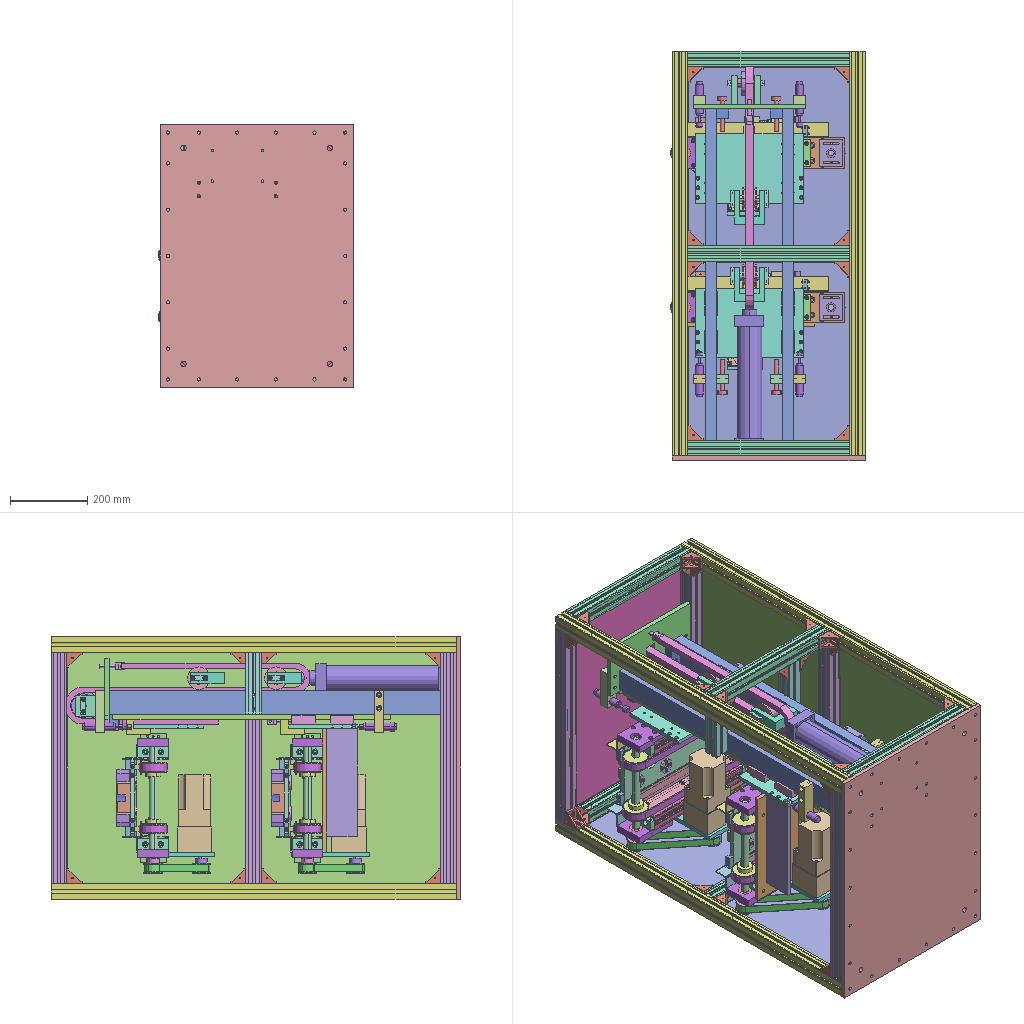Assembly | STEP file | 73 different items | 248 placed | box 503 x 1062 x 680 mm
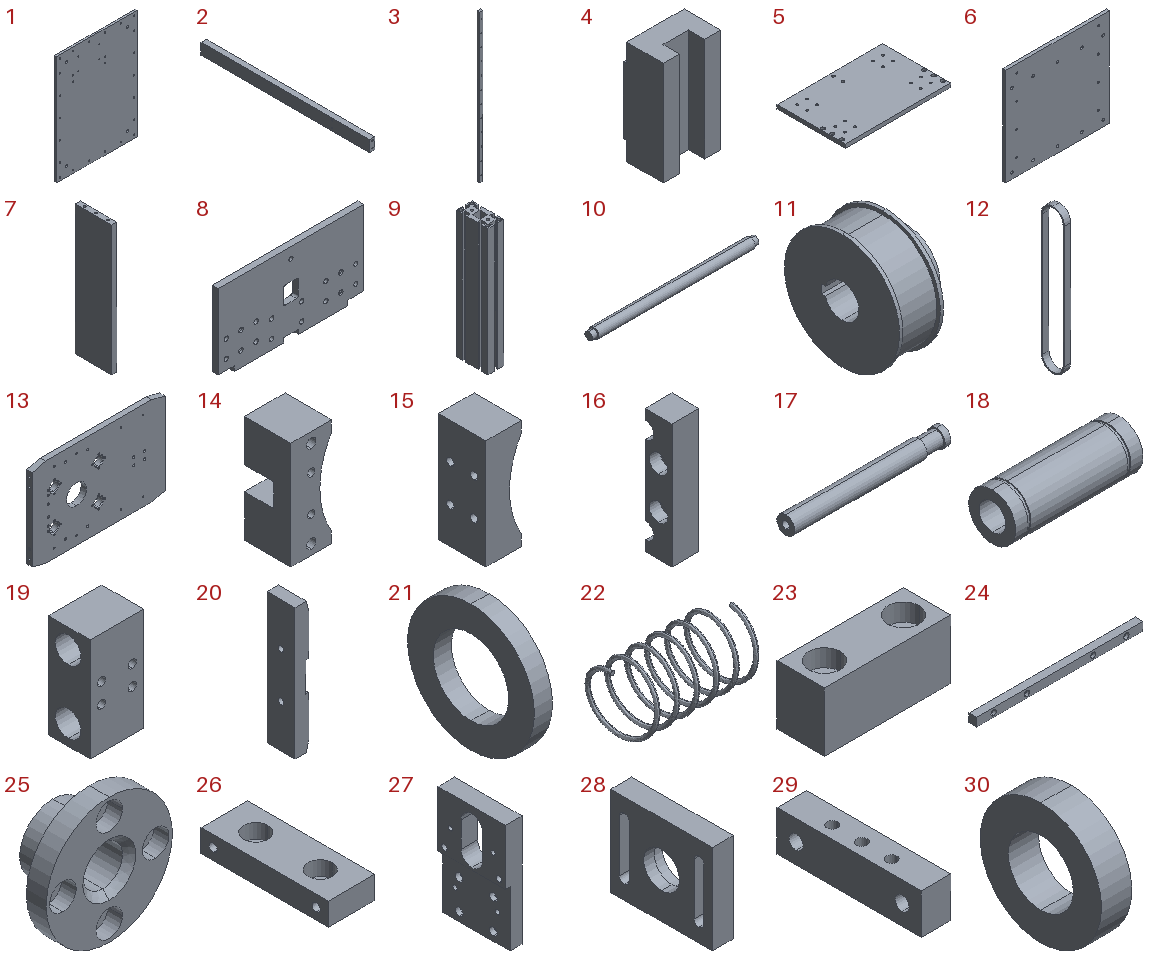Parts list (item | name | quantity | parent item | size | volume):
1 | PN_0014 (base plate) | x1 | - | 500 x 12 x 680 mm | 4053163 mm3
2 | PN_0054 (guide rail fixed plate) | x2 | - | 28 x 900 x 60 mm | 1504828 mm3
3 | PN_0064 (HGH15CA guide rail) | x2 | - | 15 x 14 x 720 mm | 146714 mm3
4 | PN_0044 (HGH15CA block) | x4 | - | 34 x 23.7 x 61.4 mm | 38690 mm3
5 | PN_0028 (connecting block) | x2 | - | 280 x 180 x 10 mm | 491440 mm3
6 | PN_0001 (support block) | x1 | - | 340 x 10 x 320 mm | 1077927 mm3
7 | PN_0070 (block) | x2 | - | 11 x 79 x 280 mm | 242077 mm3
8 | PN_0017 (fixed block) | x1 | - | 292 x 12 x 160 mm | 521488 mm3
9 | PN_0074 (cross beam) | x4 | - | 40 x 80 x 320 mm | 588947 mm3
10 | PN_0032 (secondary rotating shaft) | x2 | - | 328 x 20 x 20 mm | 99023 mm3
11 | PN_0001 (wheel) | x8 | - | 38 x 68 x 68 mm | 87974 mm3
12 | PN_0034 (conveyor belt) | x4 | - | 20 x 72 x 452 mm | 77890 mm3
13 | PN_0008 (tooling plate) | x2 | in PN_0048 (tooling assembly, return stroke) | 300 x 12 x 200 mm | 673943 mm3
14 | PN_0068 (semicircular tube block) | x2 | in PN_0048 (tooling assembly, return stroke) | 28 x 32 x 74 mm | 45440 mm3
15 | PN_0005 (movable semicircular tube block) | x2 | in PN_0045 (spring assembly) | 24 x 32 x 74 mm | 45434 mm3
16 | PN_0027 (clamp block) | x4 | in PN_0045 (spring assembly) | 16 x 16 x 74 mm | 15676 mm3
17 | PN_0025 (guide rod) | x4 | in PN_0045 (spring assembly) | 105 x 12 x 12 mm | 11156 mm3
18 | PN_0072 (bearing housing LM12LUU) | x4 | in PN_0045 (spring assembly) | 57 x 21 x 21 mm | 13212 mm3
19 | PN_0066 (guide bushing seat) | x2 | in PN_0045 (spring assembly) | 43.4 x 34 x 84 mm | 87676 mm3
20 | PN_0013 (connecting plate) | x2 | in PN_0045 (spring assembly) | 16 x 32 x 150 mm | 73689 mm3
21 | PN_0052 (stop plate) | x4 | in PN_0045 (spring assembly) | 3 x 21 x 21 mm | 670.926 mm3
22 | PN_0051 (spring) | x4 | in PN_0045 (spring assembly) | 31 x 16 x 16 mm | 222.275 mm3
23 | PN_0042 (elastic rubber) | x4 | in PN_0048 (tooling assembly, return stroke) | 32 x 12 x 15 mm | 4980 mm3
24 | PN_0040 (guide post) | x4 | in PN_0048 (tooling assembly, return stroke) | 250 x 12 x 12.5 mm | 36132 mm3
25 | PN_0059 (guide bushing) | x8 | in PN_0048 (tooling assembly, return stroke) | 38 x 17 x 38 mm | 7268 mm3
26 | PN_0053 (reinforcing block) | x8 | - | 29 x 79 x 14 mm | 27118 mm3
27 | PN_0010 (connecting plate) | x4 | - | 19.5 x 79 x 130 mm | 136895 mm3
28 | PN_0033 (secondary rotating shaft seat) | x4 | - | 14 x 68 x 60 mm | 42344 mm3
29 | PN_0047 (fixed plate) | x4 | - | 14 x 68 x 19 mm | 15184 mm3
30 | PN_0037 (ZZ6902) | x4 | - | 7 x 28 x 28 mm | 3073 mm3
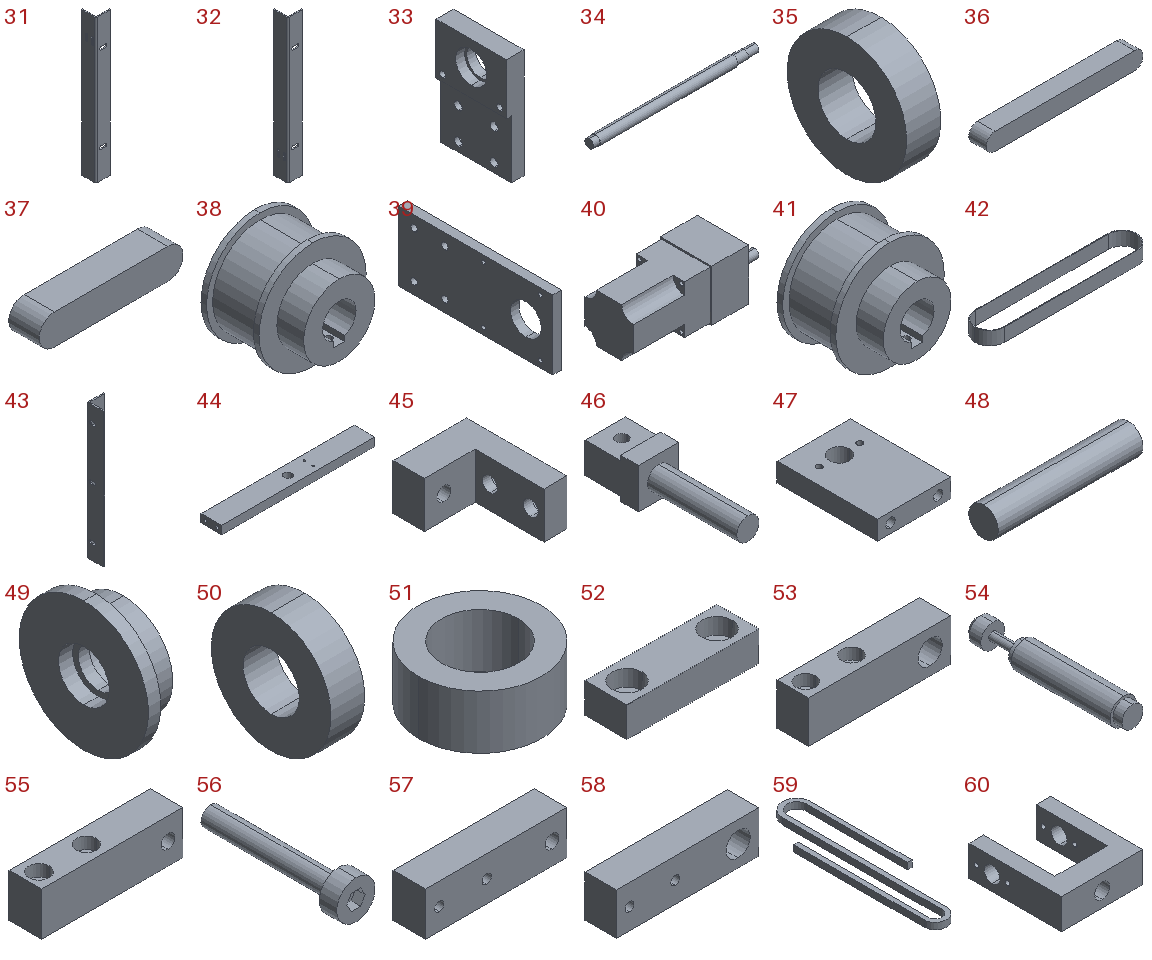31 | PN_0031 (stop side plate) | x2 | - | 40 x 40 x 400 mm | 89658 mm3
32 | PN_0067 (stop side plate) | x2 | - | 40 x 40 x 400 mm | 89658 mm3
33 | PN_0023 (connecting plate) | x4 | - | 19.5 x 79 x 122 mm | 133748 mm3
34 | PN_0012 (main rotating shaft) | x2 | - | 325 x 20 x 20 mm | 94666 mm3
35 | PN_0022 (ZZ6003) | x4 | - | 10 x 35 x 35 mm | 7351 mm3
36 | PN_0046 (5x5x40) | x8 | - | 45 x 5 x 5 mm | 1098 mm3
37 | PN_0038 (4x4x15) | x2 | - | 19 x 4 x 4 mm | 290.265 mm3
38 | PN_0055 (ATP14L075)_ATP22XL050-A-H8 | x2 | - | 48 x 38 x 48 mm | 41242 mm3
39 | PN_0021 (drive mounting plate) | x2 | - | 11 x 200 x 90 mm | 180816 mm3
40 | PN_0060 (60W.1:15) | x2 | - | 238 x 90 x 90 mm | 1379919 mm3
41 | PN_0026 (ATP14L075)_ATP22XL050-A-H8 | x2 | - | 48 x 38 x 48 mm | 40082 mm3
42 | PN_0049 (timing belt 210L, W20, Z=56) | x2 | - | 244.45 x 44.45 x 20 mm | 10730 mm3
43 | PN_0062 (belt pad block) | x4 | - | 40 x 40 x 340 mm | 77417 mm3
44 | PN_0020 (pull block) | x2 | - | 206 x 28 x 11 mm | 61677 mm3
45 | PN_0002 (connecting block) | x2 | - | 45 x 61 x 28 mm | 35599 mm3
46 | PN_0003 (hook) | x3 | - | 18 x 64 x 18 mm | 9415 mm3
47 | PN_0065 (support block) | x2 | - | 54 x 74 x 14 mm | 51598 mm3
48 | PN_0015 (shaft rod) | x1 | - | 74 x 15 x 15 mm | 13077 mm3
49 | PN_0073 (sprocket z=16,p=15.875) | x1 | - | 25 x 81.37 x 81.37 mm | 74577 mm3
50 | PN_0011 (ZZ6002) | x4 | - | 9 x 32 x 32 mm | 5648 mm3
51 | PN_0019 (stop plate) | x2 | - | 24 x 24 x 10.5 mm | 2895 mm3
52 | PN_0061 (stop block) | x6 | - | 44 x 14 x 10 mm | 5093 mm3
53 | PN_0006 (buffer fixed block) | x2 | - | 109 x 24 x 32 mm | 69208 mm3
54 | PN_0009 (hydraulic changer ACA2020) | x4 | - | 20 x 118 x 20 mm | 29167 mm3
55 | PN_0036 (positioning fixed block) | x2 | - | 104 x 24 x 32 mm | 69858 mm3
56 | PN_0057 (M12X60) | x4 | - | 24 x 91 x 24 mm | 13504 mm3
57 | PN_0030 (positioning fixed block) | x2 | - | 104 x 24 x 32 mm | 76168 mm3
58 | PN_0035 (buffer fixed block) | x2 | - | 109 x 24 x 32 mm | 75518 mm3
59 | PN_0043 (chain bar) | x1 | - | 158.46 x 636.775 x 22 mm | 522937 mm3
60 | PN_0050 (connecting block) | x2 | - | 78 x 88 x 29 mm | 91430 mm3
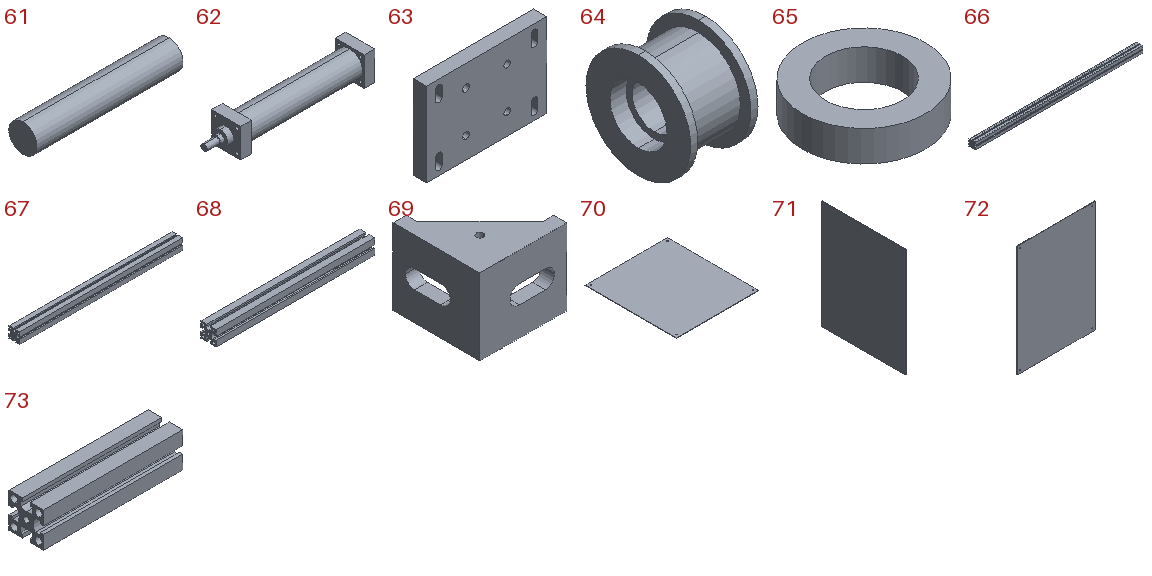61 | PN_0018 (shaft rod) | x2 | - | 78 x 15 x 15 mm | 13784 mm3
62 | PN_0029 (SC63X250) | x1 | - | 403 x 75 x 75 mm | 1293600 mm3
63 | PN_0058 (fixed plate) | x1 | - | 164 x 18 x 114 mm | 315701 mm3
64 | PN_0041 (slide wheel) | x2 | - | 38 x 59 x 59 mm | 49626 mm3
65 | PN_0016 (stop plate) | x2 | - | 24 x 24 x 6 mm | 1654 mm3
66 | PN_0024 (upright stop) | x4 | - | 1050 x 40 x 40 mm | 867444 mm3
67 | PN_0069 (cross stop) | x5 | - | 600 x 40 x 40 mm | 495706 mm3
68 | PN_0063 (cross stop) | x6 | - | 420 x 40 x 40 mm | 346994 mm3
69 | PN_0039 (4040A foot bracket) | x35 | - | 40 x 40 x 35 mm | 17755 mm3
70 | PN_0004 (cover plate) | x2 | - | 418 x 463 x 2 mm | 386911 mm3
71 | PN_0056 (cover plate) | x2 | - | 2 x 463 x 598 mm | 553591 mm3
72 | PN_0007 (cover plate) | x1 | - | 418 x 2 x 598 mm | 499771 mm3
73 | PN_0071 (reinforcing stop) | x2 | - | 160 x 40 x 40 mm | 131462 mm3
Placements (level | parent | child | x y z in mm | rotation matrix by rows):
1 | subassembly 2 | PN_0014 (base plate) | 231.231 -175.56 350.0 | 1 0 0 0 1 0 0 0 1
1 | subassembly 2 | subassembly 3 | 137.273 41.493 180.0 | 1 0 0 0 1 0 0 0 1
2 | subassembly 3 | PN_0054 (guide rail fixed plate) | -56.042 -205.053 -30.0 | 1 0 0 0 1 0 0 0 1
2 | subassembly 3 | PN_0064 (HGH15CA guide rail) | -56.042 684.947 -30.0 | 1 0 0 0 0 1 0 -1 -0
2 | subassembly 3 | PN_0044 (HGH15CA block) | -56.042 90.647 -34.3 | 1 0 0 0 0 1 0 -1 -0
2 | subassembly 3 | PN_0054 (guide rail fixed plate) | 143.958 -205.053 -30.0 | 1 0 0 0 1 0 0 0 1
2 | subassembly 3 | PN_0064 (HGH15CA guide rail) | 143.958 684.947 -30.0 | 1 0 0 0 0 1 0 -1 -0
2 | subassembly 3 | PN_0044 (HGH15CA block) | 143.958 90.647 -34.3 | 1 0 0 0 0 1 0 -1 -0
2 | subassembly 3 | PN_0028 (connecting block) | 43.958 140.647 -68.0 | 1 0 0 0 1 0 0 0 1
2 | subassembly 3 | PN_0001 (support block) | 43.958 130.647 -68.0 | 1 0 0 0 1 0 0 0 1
2 | subassembly 3 | PN_0070 (block) | 177.958 51.647 -68.0 | 1 0 0 0 1 0 0 0 1
2 | subassembly 3 | PN_0070 (block) | -90.042 51.647 -68.0 | 1 0 0 0 1 0 0 0 1
2 | subassembly 3 | PN_0017 (fixed block) | 43.958 694.947 -45.0 | 1 0 0 0 1 0 0 0 1
2 | subassembly 3 | subassembly 4 | 105.958 169.332 -414.33 | 0 0 1 0 1 0 -1 0 0
3 | subassembly 4 | PN_0074 (cross beam) | -46.33 11.315 -200.0 | 1 0 0 0 1 0 0 0 1
3 | subassembly 4 | PN_0074 (cross beam) | -286.33 11.315 -200.0 | 1 0 0 0 1 0 0 0 1
3 | subassembly 4 | PN_0032 (secondary rotating shaft) | -330.33 11.315 150.0 | 1 0 0 0 0.9618 -0.2738 0 0.2738 0.9618
3 | subassembly 4 | PN_0001 (wheel) | -73.33 11.315 150.0 | -1 0 0 0 0.9618 0.2738 0 0.2738 -0.9618
3 | subassembly 4 | PN_0034 (conveyor belt) | -86.33 11.315 150.0 | -1 0 0 0 -1 0 0 0 1
3 | subassembly 4 | PN_0001 (wheel) | -259.33 11.315 150.0 | 1 0 0 0 0.9618 -0.2738 0 0.2738 0.9618
3 | subassembly 4 | PN_0034 (conveyor belt) | -246.33 11.315 150.0 | -1 0 0 0 -1 0 0 0 1
3 | subassembly 4 | PN_0048 (tooling assembly, return stroke) | -166.33 74.53 -49.238 | 0 0 -1 0 1 0 1 0 0
4 | PN_0048 (tooling assembly, return stroke) | PN_0008 (tooling plate) | -75.335 -9.216 -0.0 | 1 0 0 0 1 0 0 0 1
4 | PN_0048 (tooling assembly, return stroke) | PN_0068 (semicircular tube block) | -153.335 12.784 -0.0 | 1 0 0 0 1 0 0 0 1
4 | PN_0048 (tooling assembly, return stroke) | PN_0045 (spring assembly) | -58.515 11.875 -0.0 | -1 0 0 0 1 0 0 0 -1
5 | PN_0045 (spring assembly) | PN_0005 (movable semicircular tube block) | -57.18 2.909 -0.0 | 1 0 0 0 1 0 0 0 1
5 | PN_0045 (spring assembly) | PN_0027 (clamp block) | -73.18 -13.091 0.0 | 1 0 0 0 1 0 0 0 1
5 | PN_0045 (spring assembly) | PN_0027 (clamp block) | -73.18 18.909 -0.0 | 1 0 0 0 -1 0 0 0 -1
5 | PN_0045 (spring assembly) | PN_0025 (guide rod) | -162.18 2.909 -26.0 | 1 0 0 0 0.9992 -0.03879 0 0.03879 0.9992
5 | PN_0045 (spring assembly) | PN_0025 (guide rod) | -162.18 2.909 26.0 | 1 0 0 0 0.4218 -0.9067 0 0.9067 0.4218
5 | PN_0045 (spring assembly) | PN_0072 (bearing housing LM12LUU) | -153.18 2.909 -26.0 | 1 0 0 0 1 0 0 0 1
5 | PN_0045 (spring assembly) | PN_0072 (bearing housing LM12LUU) | -153.18 2.909 26.0 | 1 0 0 0 1 0 0 0 1
5 | PN_0045 (spring assembly) | PN_0066 (guide bushing seat) | -124.68 -15.091 -0.0 | 1 0 0 0 1 0 0 0 1
5 | PN_0045 (spring assembly) | PN_0013 (connecting plate) | -178.18 2.909 -0.0 | 1 0 0 0 1 0 0 0 1
5 | PN_0045 (spring assembly) | PN_0052 (stop plate) | -96.18 2.909 26.0 | 1 0 0 0 1 0 0 0 1
5 | PN_0045 (spring assembly) | PN_0052 (stop plate) | -96.18 2.909 -26.0 | 1 0 0 0 1 0 0 0 1
5 | PN_0045 (spring assembly) | PN_0051 (spring) | -97.732 2.909 26.0 | 1 0 0 0 1 0 0 0 1
5 | PN_0045 (spring assembly) | PN_0051 (spring) | -97.081 2.909 -26.0 | 1 0 0 0 0.9742 -0.2257 0 0.2257 0.9742
4 | PN_0048 (tooling assembly, return stroke) | PN_0042 (elastic rubber) | -175.335 -9.216 -70.0 | 0 0 -1 0 1 0 1 0 0
4 | PN_0048 (tooling assembly, return stroke) | PN_0042 (elastic rubber) | -175.335 -9.216 70.0 | 0 0 -1 0 1 0 1 0 0
4 | PN_0048 (tooling assembly, return stroke) | PN_0040 (guide post) | -25.335 -27.215 80.0 | 1 0 0 0 1 0 0 0 1
4 | PN_0048 (tooling assembly, return stroke) | PN_0040 (guide post) | -25.335 -27.215 -80.0 | 1 0 0 0 1 0 0 0 1
4 | PN_0048 (tooling assembly, return stroke) | PN_0059 (guide bushing) | -125.335 -21.215 40.0 | 1 0 0 0 1 0 0 0 1
4 | PN_0048 (tooling assembly, return stroke) | PN_0059 (guide bushing) | -125.335 -21.215 -40.0 | 1 0 0 0 1 0 0 0 1
4 | PN_0048 (tooling assembly, return stroke) | PN_0059 (guide bushing) | -25.335 -21.215 40.0 | 1 0 0 0 1 0 0 0 1
4 | PN_0048 (tooling assembly, return stroke) | PN_0059 (guide bushing) | -25.335 -21.215 -40.0 | 1 0 0 0 1 0 0 0 1
3 | subassembly 4 | PN_0053 (reinforcing block) | -46.33 11.315 120.0 | 1 0 0 0 1 0 0 0 1
3 | subassembly 4 | PN_0053 (reinforcing block) | -286.33 11.315 120.0 | 1 0 0 0 1 0 0 0 1
3 | subassembly 4 | PN_0053 (reinforcing block) | -46.33 11.315 -200.0 | -1 0 0 0 1 0 0 0 -1
3 | subassembly 4 | PN_0053 (reinforcing block) | -286.33 11.315 -200.0 | -1 0 0 0 1 0 0 0 -1
3 | subassembly 4 | subassembly 5 | -332.66 22.63 -80.0 | -1 0 0 0 -1 0 0 0 1
4 | subassembly 5 | PN_0010 (connecting plate) | -31.83 11.315 135.0 | 1 0 0 0 1 0 0 0 1
4 | subassembly 5 | PN_0033 (secondary rotating shaft seat) | -5.33 11.315 230.0 | -1 0 0 0 1 0 0 0 -1
4 | subassembly 5 | PN_0047 (fixed plate) | -5.33 11.315 167.0 | 1 0 0 0 1 0 0 0 1
4 | subassembly 5 | PN_0037 (ZZ6902) | -12.33 11.315 230.0 | 1 0 0 0 1 0 0 0 1
3 | subassembly 4 | subassembly 5 | -0.0 -0.0 -80.0 | 1 0 0 0 1 0 0 0 1
4 | subassembly 5 | PN_0010 (connecting plate) | -31.83 11.315 135.0 | 1 0 0 0 1 0 0 0 1
4 | subassembly 5 | PN_0033 (secondary rotating shaft seat) | -5.33 11.315 230.0 | -1 0 0 0 1 0 0 0 -1
4 | subassembly 5 | PN_0047 (fixed plate) | -5.33 11.315 167.0 | 1 0 0 0 1 0 0 0 1
4 | subassembly 5 | PN_0037 (ZZ6902) | -12.33 11.315 230.0 | 1 0 0 0 1 0 0 0 1
3 | subassembly 4 | PN_0031 (stop side plate) | -66.33 51.315 143.0 | 1 0 0 0 1 0 0 0 1
3 | subassembly 4 | PN_0067 (stop side plate) | -266.33 51.315 -257.0 | -1 0 0 0 1 0 0 0 -1
3 | subassembly 4 | PN_0023 (connecting plate) | -31.83 11.315 -135.0 | 1 0 0 0 -1 0 0 0 -1
3 | subassembly 4 | PN_0023 (connecting plate) | -300.83 11.315 -135.0 | -1 0 0 0 1 0 0 0 -1
3 | subassembly 4 | PN_0012 (main rotating shaft) | -312.83 11.315 -230.0 | 1 0 0 0 0.9232 0.3844 0 -0.3844 0.9232
3 | subassembly 4 | PN_0022 (ZZ6003) | -310.83 11.315 -230.0 | 1 0 0 0 1 0 0 0 1
3 | subassembly 4 | PN_0022 (ZZ6003) | -31.83 11.315 -230.0 | 1 0 0 0 1 0 0 0 1
3 | subassembly 4 | PN_0046 (5x5x40) | -240.33 18.047 151.917 | 1 0 0 0 0.9618 -0.2738 0 0.2738 0.9618
3 | subassembly 4 | PN_0046 (5x5x40) | -92.33 18.047 151.917 | 1 0 0 0 0.9618 -0.2738 0 0.2738 0.9618
3 | subassembly 4 | PN_0046 (5x5x40) | -240.33 17.777 -232.69 | 1 0 0 0 0.9232 0.3844 0 -0.3844 0.9232
3 | subassembly 4 | PN_0046 (5x5x40) | -92.33 17.777 -232.69 | 1 0 0 0 0.9232 0.3844 0 -0.3844 0.9232
3 | subassembly 4 | PN_0001 (wheel) | -73.33 11.315 -230.0 | -1 0 0 0 0.9232 -0.3844 0 -0.3844 -0.9232
3 | subassembly 4 | PN_0001 (wheel) | -259.33 11.315 -230.0 | 1 0 0 0 0.9232 0.3844 0 -0.3844 0.9232
3 | subassembly 4 | PN_0038 (4x4x15) | 0.6702 15.931 -231.922 | 1 0 0 0 0.9232 0.3844 0 -0.3844 0.9232
3 | subassembly 4 | PN_0055 (ATP14L075)_ATP22XL050-A-H8 | 4.67 11.315 -230.0 | 0 1 0 0.8409 0 0.5412 0.5412 0 -0.8409
3 | subassembly 4 | subassembly 6 | 16.937 -58.379 -73.875 | 1 0 0 0 1 0 0 0 1
4 | subassembly 6 | PN_0021 (drive mounting plate) | -37.767 -90.306 -0.0 | 1 0 0 0 1 0 0 0 1
4 | subassembly 6 | PN_0060 (60W.1:15) | -108.267 -37.306 -0.0 | 1 0 0 0 1 0 0 0 1
4 | subassembly 6 | PN_0026 (ATP14L075)_ATP22XL050-A-H8 | -12.267 -55.306 0.0 | 0 1 0 -0.1427 0 -0.9898 -0.9898 0 0.1427
3 | subassembly 4 | PN_0049 (timing belt 210L, W20, Z=56) | 15.217 -51.185 -151.938 | 0 0 1 0.625 0.7806 0 -0.7806 0.625 0
3 | subassembly 4 | PN_0062 (belt pad block) | -266.33 3.315 130.0 | 1 0 0 0 1 0 0 0 1
3 | subassembly 4 | PN_0062 (belt pad block) | -66.33 3.315 -210.0 | -1 0 0 0 1 0 0 0 -1
3 | subassembly 4 | PN_0020 (pull block) | -169.33 55.315 82.5 | 1 0 0 0 1 0 0 0 1
2 | subassembly 3 | PN_0044 (HGH15CA block) | -56.042 190.647 -34.3 | 1 0 0 0 0 1 0 -1 -0
2 | subassembly 3 | PN_0044 (HGH15CA block) | 143.958 190.647 -34.3 | 1 0 0 0 0 1 0 -1 -0
2 | subassembly 3 | PN_0002 (connecting block) | 43.958 188.647 -82.0 | 0 0 1 0 1 0 -1 0 0
2 | subassembly 3 | PN_0003 (hook) | 43.958 220.647 -49.0 | 0 0 1 0 1 0 -1 0 0
2 | subassembly 3 | subassembly 7 | 5.358 752.51 1.624 | 0 0 -1 0 1 0 1 0 0
3 | subassembly 7 | PN_0065 (support block) | -9.939 -45.563 -0.0 | 1 0 0 0 1 0 0 0 1
3 | subassembly 7 | PN_0065 (support block) | -9.939 -45.563 -60.0 | 1 0 0 0 1 0 0 0 1
3 | subassembly 7 | PN_0015 (shaft rod) | -9.939 9.437 -30.0 | 0 -0.03289 0.9995 0 0.9995 0.03289 -1 0 0
3 | subassembly 7 | subassembly 8 | -9.323 17.636 -38.04 | 0 0.07491 -0.9972 0 0.9972 0.07491 1 0 0
4 | subassembly 8 | PN_0073 (sprocket z=16,p=15.875) | -4.46 -8.221 0.0 | 1 0 0 0 0.8869 -0.4619 0 0.4619 0.8869
4 | subassembly 8 | PN_0011 (ZZ6002) | 11.54 -8.221 0.0 | 1 0 0 0 1 0 0 0 1
4 | subassembly 8 | PN_0011 (ZZ6002) | -4.46 -8.221 0.0 | 1 0 0 0 1 0 0 0 1
3 | subassembly 7 | PN_0019 (stop plate) | -9.939 9.437 -17.5 | 1 0 0 0 1 0 0 0 1
3 | subassembly 7 | PN_0019 (stop plate) | -9.939 9.437 -53.0 | 0.9993 0.03637 0 -0.03637 0.9993 0 0 0 1
3 | subassembly 7 | PN_0061 (stop block) | -9.939 9.437 7.0 | 1 0 0 0 1 0 0 0 1
3 | subassembly 7 | PN_0061 (stop block) | -9.939 9.437 -67.0 | -1 0 0 0 1 0 0 0 -1
2 | subassembly 3 | PN_0003 (hook) | 43.958 718.947 93.5 | 0 0 -1 0 -1 0 -1 0 0
2 | subassembly 3 | subassembly 9 | 173.958 -10.863 -72.058 | 0 0 1 0 1 0 -1 0 0
3 | subassembly 9 | PN_0006 (buffer fixed block) | -102.058 5.81 -0.0 | 1 0 0 0 1 0 0 0 1
3 | subassembly 9 | PN_0009 (hydraulic changer ACA2020) | -9.058 -40.34 -0.0 | 1 0 0 0 1 0 0 0 1
2 | subassembly 3 | subassembly 10 | 113.958 -3.218 -34.749 | 0 0 -1 0 -1 0 -1 0 -0
3 | subassembly 10 | PN_0036 (positioning fixed block) | -64.749 1.835 -0.0 | 1 0 0 0 1 0 0 0 1
3 | subassembly 10 | PN_0057 (M12X60) | 28.251 43.274 -0.0 | -0.9457 0 0.3251 0 -1 0 0.3251 0 0.9457
2 | subassembly 3 | subassembly 9 | -86.042 -10.863 -72.058 | 0 0 1 0 1 0 -1 0 0
3 | subassembly 9 | PN_0006 (buffer fixed block) | -102.058 5.81 -0.0 | 1 0 0 0 1 0 0 0 1
3 | subassembly 9 | PN_0009 (hydraulic changer ACA2020) | -9.058 -40.34 -0.0 | 1 0 0 0 1 0 0 0 1
2 | subassembly 3 | subassembly 10 | -26.042 -3.218 -34.749 | 0 0 -1 0 -1 0 -1 0 0
3 | subassembly 10 | PN_0036 (positioning fixed block) | -64.749 1.835 -0.0 | 1 0 0 0 1 0 0 0 1
3 | subassembly 10 | PN_0057 (M12X60) | 28.251 43.274 -0.0 | -0.9457 0 0.3251 0 -1 0 0.3251 0 0.9457
2 | subassembly 3 | subassembly 11 | 113.958 684.782 -34.749 | 0 0 -1 0 -1 0 -1 0 0
3 | subassembly 11 | PN_0030 (positioning fixed block) | -64.749 1.835 -0.0 | 1 0 0 0 1 0 0 0 1
3 | subassembly 11 | PN_0057 (M12X60) | 28.251 -42.058 0.0 | 0.9854 0 0.1701 0 1 0 -0.1701 0 0.9854
2 | subassembly 3 | subassembly 11 | -26.042 684.782 -34.749 | 0 0 -1 0 -1 0 -1 0 0
3 | subassembly 11 | PN_0030 (positioning fixed block) | -64.749 1.835 -0.0 | 1 0 0 0 1 0 0 0 1
3 | subassembly 11 | PN_0057 (M12X60) | 28.251 -42.058 0.0 | 0.9854 0 0.1701 0 1 0 -0.1701 0 0.9854
2 | subassembly 3 | subassembly 12 | 173.958 724.757 -72.058 | 0 0 -1 0 -1 0 -1 0 0
3 | subassembly 12 | PN_0035 (buffer fixed block) | -102.058 5.81 -0.0 | 1 0 0 0 1 0 0 0 1
3 | subassembly 12 | PN_0009 (hydraulic changer ACA2020) | -9.058 -40.34 -0.0 | 1 0 0 0 1 0 0 0 1
2 | subassembly 3 | subassembly 12 | -86.042 724.757 -72.058 | 0 0 -1 0 -1 0 -1 0 0
3 | subassembly 12 | PN_0035 (buffer fixed block) | -102.058 5.81 -0.0 | 1 0 0 0 1 0 0 0 1
3 | subassembly 12 | PN_0009 (hydraulic changer ACA2020) | -9.058 -40.34 -0.0 | 1 0 0 0 1 0 0 0 1
2 | subassembly 3 | PN_0002 (connecting block) | 43.958 588.647 -82.0 | 0 0 1 0 1 0 -1 0 0
2 | subassembly 3 | PN_0003 (hook) | 43.958 620.647 -49.0 | 0 0 1 0 1 0 -1 0 0
2 | subassembly 3 | PN_0028 (connecting block) | 43.958 540.647 -68.0 | 1 0 0 0 1 0 0 0 1
2 | subassembly 3 | subassembly 4 | 105.958 569.332 -414.33 | 0 0 1 0 1 0 -1 0 0
3 | subassembly 4 | PN_0074 (cross beam) | -46.33 11.315 -200.0 | 1 0 0 0 1 0 0 0 1
3 | subassembly 4 | PN_0074 (cross beam) | -286.33 11.315 -200.0 | 1 0 0 0 1 0 0 0 1
3 | subassembly 4 | PN_0032 (secondary rotating shaft) | -330.33 11.315 150.0 | 1 0 0 0 0.9618 -0.2738 0 0.2738 0.9618
3 | subassembly 4 | PN_0001 (wheel) | -73.33 11.315 150.0 | -1 0 0 0 0.9618 0.2738 0 0.2738 -0.9618
3 | subassembly 4 | PN_0034 (conveyor belt) | -86.33 11.315 150.0 | -1 0 0 0 -1 0 0 0 1
3 | subassembly 4 | PN_0001 (wheel) | -259.33 11.315 150.0 | 1 0 0 0 0.9618 -0.2738 0 0.2738 0.9618
3 | subassembly 4 | PN_0034 (conveyor belt) | -246.33 11.315 150.0 | -1 0 0 0 -1 0 0 0 1
3 | subassembly 4 | PN_0048 (tooling assembly, return stroke) | -166.33 74.53 -49.238 | 0 0 -1 0 1 0 1 0 0
4 | PN_0048 (tooling assembly, return stroke) | PN_0008 (tooling plate) | -75.335 -9.216 -0.0 | 1 0 0 0 1 0 0 0 1
4 | PN_0048 (tooling assembly, return stroke) | PN_0068 (semicircular tube block) | -153.335 12.784 -0.0 | 1 0 0 0 1 0 0 0 1
4 | PN_0048 (tooling assembly, return stroke) | PN_0045 (spring assembly) | -58.515 11.875 -0.0 | -1 0 0 0 1 0 0 0 -1
5 | PN_0045 (spring assembly) | PN_0005 (movable semicircular tube block) | -57.18 2.909 -0.0 | 1 0 0 0 1 0 0 0 1
5 | PN_0045 (spring assembly) | PN_0027 (clamp block) | -73.18 -13.091 0.0 | 1 0 0 0 1 0 0 0 1
5 | PN_0045 (spring assembly) | PN_0027 (clamp block) | -73.18 18.909 -0.0 | 1 0 0 0 -1 0 0 0 -1
5 | PN_0045 (spring assembly) | PN_0025 (guide rod) | -162.18 2.909 -26.0 | 1 0 0 0 0.9992 -0.03879 0 0.03879 0.9992
5 | PN_0045 (spring assembly) | PN_0025 (guide rod) | -162.18 2.909 26.0 | 1 0 0 0 0.4218 -0.9067 0 0.9067 0.4218
5 | PN_0045 (spring assembly) | PN_0072 (bearing housing LM12LUU) | -153.18 2.909 -26.0 | 1 0 0 0 1 0 0 0 1
5 | PN_0045 (spring assembly) | PN_0072 (bearing housing LM12LUU) | -153.18 2.909 26.0 | 1 0 0 0 1 0 0 0 1
5 | PN_0045 (spring assembly) | PN_0066 (guide bushing seat) | -124.68 -15.091 -0.0 | 1 0 0 0 1 0 0 0 1
5 | PN_0045 (spring assembly) | PN_0013 (connecting plate) | -178.18 2.909 -0.0 | 1 0 0 0 1 0 0 0 1
5 | PN_0045 (spring assembly) | PN_0052 (stop plate) | -96.18 2.909 26.0 | 1 0 0 0 1 0 0 0 1
5 | PN_0045 (spring assembly) | PN_0052 (stop plate) | -96.18 2.909 -26.0 | 1 0 0 0 1 0 0 0 1
5 | PN_0045 (spring assembly) | PN_0051 (spring) | -97.732 2.909 26.0 | 1 0 0 0 1 0 0 0 1
5 | PN_0045 (spring assembly) | PN_0051 (spring) | -97.081 2.909 -26.0 | 1 0 0 0 0.9742 -0.2257 0 0.2257 0.9742
4 | PN_0048 (tooling assembly, return stroke) | PN_0042 (elastic rubber) | -175.335 -9.216 -70.0 | 0 0 -1 0 1 0 1 0 0
4 | PN_0048 (tooling assembly, return stroke) | PN_0042 (elastic rubber) | -175.335 -9.216 70.0 | 0 0 -1 0 1 0 1 0 0
4 | PN_0048 (tooling assembly, return stroke) | PN_0040 (guide post) | -25.335 -27.215 80.0 | 1 0 0 0 1 0 0 0 1
4 | PN_0048 (tooling assembly, return stroke) | PN_0040 (guide post) | -25.335 -27.215 -80.0 | 1 0 0 0 1 0 0 0 1
4 | PN_0048 (tooling assembly, return stroke) | PN_0059 (guide bushing) | -125.335 -21.215 40.0 | 1 0 0 0 1 0 0 0 1
4 | PN_0048 (tooling assembly, return stroke) | PN_0059 (guide bushing) | -125.335 -21.215 -40.0 | 1 0 0 0 1 0 0 0 1
4 | PN_0048 (tooling assembly, return stroke) | PN_0059 (guide bushing) | -25.335 -21.215 40.0 | 1 0 0 0 1 0 0 0 1
4 | PN_0048 (tooling assembly, return stroke) | PN_0059 (guide bushing) | -25.335 -21.215 -40.0 | 1 0 0 0 1 0 0 0 1
3 | subassembly 4 | PN_0053 (reinforcing block) | -46.33 11.315 120.0 | 1 0 0 0 1 0 0 0 1
3 | subassembly 4 | PN_0053 (reinforcing block) | -286.33 11.315 120.0 | 1 0 0 0 1 0 0 0 1
3 | subassembly 4 | PN_0053 (reinforcing block) | -46.33 11.315 -200.0 | -1 0 0 0 1 0 0 0 -1
3 | subassembly 4 | PN_0053 (reinforcing block) | -286.33 11.315 -200.0 | -1 0 0 0 1 0 0 0 -1
3 | subassembly 4 | subassembly 5 | -332.66 22.63 -80.0 | -1 0 0 0 -1 0 0 0 1
4 | subassembly 5 | PN_0010 (connecting plate) | -31.83 11.315 135.0 | 1 0 0 0 1 0 0 0 1
4 | subassembly 5 | PN_0033 (secondary rotating shaft seat) | -5.33 11.315 230.0 | -1 0 0 0 1 0 0 0 -1
4 | subassembly 5 | PN_0047 (fixed plate) | -5.33 11.315 167.0 | 1 0 0 0 1 0 0 0 1
4 | subassembly 5 | PN_0037 (ZZ6902) | -12.33 11.315 230.0 | 1 0 0 0 1 0 0 0 1
3 | subassembly 4 | subassembly 5 | -0.0 -0.0 -80.0 | 1 0 0 0 1 0 0 0 1
4 | subassembly 5 | PN_0010 (connecting plate) | -31.83 11.315 135.0 | 1 0 0 0 1 0 0 0 1
4 | subassembly 5 | PN_0033 (secondary rotating shaft seat) | -5.33 11.315 230.0 | -1 0 0 0 1 0 0 0 -1
4 | subassembly 5 | PN_0047 (fixed plate) | -5.33 11.315 167.0 | 1 0 0 0 1 0 0 0 1
4 | subassembly 5 | PN_0037 (ZZ6902) | -12.33 11.315 230.0 | 1 0 0 0 1 0 0 0 1
3 | subassembly 4 | PN_0031 (stop side plate) | -66.33 51.315 143.0 | 1 0 0 0 1 0 0 0 1
3 | subassembly 4 | PN_0067 (stop side plate) | -266.33 51.315 -257.0 | -1 0 0 0 1 0 0 0 -1
3 | subassembly 4 | PN_0023 (connecting plate) | -31.83 11.315 -135.0 | 1 0 0 0 -1 0 0 0 -1
3 | subassembly 4 | PN_0023 (connecting plate) | -300.83 11.315 -135.0 | -1 0 0 0 1 0 0 0 -1
3 | subassembly 4 | PN_0012 (main rotating shaft) | -312.83 11.315 -230.0 | 1 0 0 0 0.9232 0.3844 0 -0.3844 0.9232
3 | subassembly 4 | PN_0022 (ZZ6003) | -310.83 11.315 -230.0 | 1 0 0 0 1 0 0 0 1
3 | subassembly 4 | PN_0022 (ZZ6003) | -31.83 11.315 -230.0 | 1 0 0 0 1 0 0 0 1
3 | subassembly 4 | PN_0046 (5x5x40) | -240.33 18.047 151.917 | 1 0 0 0 0.9618 -0.2738 0 0.2738 0.9618
3 | subassembly 4 | PN_0046 (5x5x40) | -92.33 18.047 151.917 | 1 0 0 0 0.9618 -0.2738 0 0.2738 0.9618
3 | subassembly 4 | PN_0046 (5x5x40) | -240.33 17.777 -232.69 | 1 0 0 0 0.9232 0.3844 0 -0.3844 0.9232
3 | subassembly 4 | PN_0046 (5x5x40) | -92.33 17.777 -232.69 | 1 0 0 0 0.9232 0.3844 0 -0.3844 0.9232
3 | subassembly 4 | PN_0001 (wheel) | -73.33 11.315 -230.0 | -1 0 0 0 0.9232 -0.3844 0 -0.3844 -0.9232
3 | subassembly 4 | PN_0001 (wheel) | -259.33 11.315 -230.0 | 1 0 0 0 0.9232 0.3844 0 -0.3844 0.9232
3 | subassembly 4 | PN_0038 (4x4x15) | 0.6702 15.931 -231.922 | 1 0 0 0 0.9232 0.3844 0 -0.3844 0.9232
3 | subassembly 4 | PN_0055 (ATP14L075)_ATP22XL050-A-H8 | 4.67 11.315 -230.0 | 0 1 0 0.8409 0 0.5412 0.5412 0 -0.8409
3 | subassembly 4 | subassembly 6 | 16.937 -58.379 -73.875 | 1 0 0 0 1 0 0 0 1
4 | subassembly 6 | PN_0021 (drive mounting plate) | -37.767 -90.306 -0.0 | 1 0 0 0 1 0 0 0 1
4 | subassembly 6 | PN_0060 (60W.1:15) | -108.267 -37.306 -0.0 | 1 0 0 0 1 0 0 0 1
4 | subassembly 6 | PN_0026 (ATP14L075)_ATP22XL050-A-H8 | -12.267 -55.306 0.0 | 0 1 0 -0.1427 0 -0.9898 -0.9898 0 0.1427
3 | subassembly 4 | PN_0049 (timing belt 210L, W20, Z=56) | 15.217 -51.185 -151.938 | 0 0 1 0.625 0.7806 0 -0.7806 0.625 0
3 | subassembly 4 | PN_0062 (belt pad block) | -266.33 3.315 130.0 | 1 0 0 0 1 0 0 0 1
3 | subassembly 4 | PN_0062 (belt pad block) | -66.33 3.315 -210.0 | -1 0 0 0 1 0 0 0 -1
3 | subassembly 4 | PN_0020 (pull block) | -169.33 55.315 82.5 | 1 0 0 0 1 0 0 0 1
1 | subassembly 2 | PN_0043 (chain bar) | 181.231 103.441 171.685 | 0 0 1 0 1 0 -1 0 0
1 | subassembly 2 | subassembly 13 | 231.761 295.662 243.0 | 1 0 0 0 1 0 0 0 1
2 | subassembly 13 | PN_0050 (connecting block) | -50.53 -58.221 -0.0 | 1 0 0 0 1 0 0 0 1
2 | subassembly 13 | PN_0018 (shaft rod) | -50.53 7.779 0.0 | 1 0 0 0 -0.9998 -0.01988 0 0.01988 -0.9998
2 | subassembly 13 | PN_0029 (SC63X250) | -50.53 -413.721 -0.0 | 0 1 0 -1 0 0 0 0 1
2 | subassembly 13 | PN_0058 (fixed plate) | -50.53 -450.221 -0.0 | 1 0 0 0 1 0 0 0 1
2 | subassembly 13 | PN_0061 (stop block) | -89.53 7.779 -0.0 | 0 0 -1 -1 0 0 0 1 0
2 | subassembly 13 | PN_0061 (stop block) | -11.53 7.779 0.0 | 0 0 1 -1 0 0 0 -1 0
2 | subassembly 13 | PN_0041 (slide wheel) | -69.53 7.779 0.0 | 1 0 0 0 0.9396 -0.3422 0 0.3422 0.9396
2 | subassembly 13 | PN_0011 (ZZ6002) | -40.53 7.779 -0.0 | 1 0 0 0 1 0 0 0 1
2 | subassembly 13 | PN_0011 (ZZ6002) | -69.53 7.779 -0.0 | 1 0 0 0 1 0 0 0 1
2 | subassembly 13 | PN_0016 (stop plate) | -25.53 7.779 -0.0 | 0 0 -1 0 1 0 1 0 0
2 | subassembly 13 | PN_0016 (stop plate) | -69.53 7.779 -0.0 | 0 0 -1 0.4887 0.8725 0 0.8725 -0.4887 0
2 | subassembly 13 | PN_0018 (shaft rod) | -50.53 207.779 -0.0 | 1 0 0 0 -0.9998 -0.01988 0 0.01988 -0.9998
2 | subassembly 13 | PN_0061 (stop block) | -89.53 207.779 -0.0 | 0 0 -1 -1 0 0 0 1 0
2 | subassembly 13 | PN_0061 (stop block) | -11.53 207.779 0.0 | 0 0 1 -1 0 0 0 -1 0
2 | subassembly 13 | PN_0050 (connecting block) | -50.53 141.779 -0.0 | 1 0 0 0 1 0 0 0 1
2 | subassembly 13 | PN_0041 (slide wheel) | -69.53 207.779 0.0 | 1 0 0 0 0.9396 -0.3422 0 0.3422 0.9396
1 | subassembly 2 | subassembly 14 | 0.0 190.0 -0.0 | 1 0 0 0 1 0 0 0 1
2 | subassembly 14 | PN_0024 (upright stop) | 461.231 696.441 330.0 | 0 1 0 -1 0 0 0 0 1
2 | subassembly 14 | PN_0024 (upright stop) | 461.231 696.441 -310.0 | 0 1 0 -1 0 0 0 0 1
2 | subassembly 14 | PN_0024 (upright stop) | 1.231 696.441 -310.0 | 0 1 0 -1 0 0 0 0 1
2 | subassembly 14 | PN_0024 (upright stop) | 1.231 696.441 330.0 | 0 1 0 -1 0 0 0 0 1
2 | subassembly 14 | PN_0069 (cross stop) | 461.231 676.441 310.0 | 0 0 1 0 1 0 -1 0 0
2 | subassembly 14 | PN_0069 (cross stop) | 1.231 676.441 310.0 | 0 0 1 0 1 0 -1 0 0
2 | subassembly 14 | PN_0063 (cross stop) | 21.231 676.441 -310.0 | 1 0 0 0 1 0 0 0 1
2 | subassembly 14 | PN_0063 (cross stop) | 21.231 676.441 330.0 | 1 0 0 0 1 0 0 0 1
2 | subassembly 14 | PN_0063 (cross stop) | 21.231 -333.56 -310.0 | 1 0 0 0 1 0 0 0 1
2 | subassembly 14 | PN_0069 (cross stop) | 461.231 -333.56 310.0 | 0 0 1 0 1 0 -1 0 0
2 | subassembly 14 | PN_0069 (cross stop) | 1.231 -333.56 310.0 | 0 0 1 0 1 0 -1 0 0
2 | subassembly 14 | PN_0063 (cross stop) | 21.231 -333.56 330.0 | 1 0 0 0 1 0 0 0 1
2 | subassembly 14 | PN_0039 (4040A foot bracket) | 461.231 -313.56 -290.0 | 0 0 -1 0 1 0 1 0 -0
2 | subassembly 14 | PN_0039 (4040A foot bracket) | 461.231 -313.56 310.0 | 0 0 1 0 1 0 -1 0 0
2 | subassembly 14 | PN_0039 (4040A foot bracket) | 461.231 656.441 310.0 | 0 0 -1 0 -1 0 -1 0 0
2 | subassembly 14 | PN_0039 (4040A foot bracket) | 461.231 656.441 -290.0 | 0 0 1 0 -1 0 1 0 0
2 | subassembly 14 | PN_0039 (4040A foot bracket) | 1.231 656.441 -290.0 | 0 0 1 0 -1 0 1 0 0
2 | subassembly 14 | PN_0039 (4040A foot bracket) | 1.231 -313.56 -290.0 | 0 0 1 1 0 0 0 1 0
2 | subassembly 14 | PN_0039 (4040A foot bracket) | 1.231 -313.56 310.0 | 0 0 -1 1 0 0 0 -1 -0
2 | subassembly 14 | PN_0039 (4040A foot bracket) | 1.231 656.441 310.0 | 0 0 -1 0 -1 0 -1 0 -0
2 | subassembly 14 | PN_0039 (4040A foot bracket) | 21.231 -313.56 330.0 | 0 1 0 1 0 0 0 0 -1
2 | subassembly 14 | PN_0039 (4040A foot bracket) | 441.231 -313.56 330.0 | 0 -1 0 1 0 0 0 0 1
2 | subassembly 14 | PN_0039 (4040A foot bracket) | 441.231 656.441 330.0 | -1 0 0 0 -1 0 0 0 1
2 | subassembly 14 | PN_0039 (4040A foot bracket) | 21.231 656.441 330.0 | 1 0 0 0 -1 0 0 0 -1
2 | subassembly 14 | PN_0039 (4040A foot bracket) | 21.231 656.441 -310.0 | 1 0 0 0 -1 0 0 0 -1
2 | subassembly 14 | PN_0039 (4040A foot bracket) | 21.231 -313.56 -310.0 | 0 1 0 1 0 0 0 0 -1
2 | subassembly 14 | PN_0039 (4040A foot bracket) | 441.231 -313.56 -310.0 | -1 0 0 0 1 0 0 0 -1
2 | subassembly 14 | PN_0039 (4040A foot bracket) | 441.231 656.441 -310.0 | 0 -1 0 -1 0 0 0 0 -1
2 | subassembly 14 | PN_0069 (cross stop) | 461.231 171.44 310.0 | 0 0 1 0 1 0 -1 0 0
2 | subassembly 14 | PN_0063 (cross stop) | 21.231 171.44 330.0 | 1 0 0 0 1 0 0 0 1
2 | subassembly 14 | PN_0063 (cross stop) | 21.231 171.44 -310.0 | 1 0 0 0 1 0 0 0 1
2 | subassembly 14 | PN_0039 (4040A foot bracket) | 461.231 151.44 -290.0 | 0 0 -1 -1 0 0 0 1 -0
2 | subassembly 14 | PN_0039 (4040A foot bracket) | 461.231 151.44 310.0 | 0 0 -1 0 -1 0 -1 0 -0
2 | subassembly 14 | PN_0039 (4040A foot bracket) | 461.231 191.44 310.0 | 0 0 1 0 1 0 -1 0 0
2 | subassembly 14 | PN_0039 (4040A foot bracket) | 461.231 191.44 -290.0 | 0 0 -1 0 1 0 1 0 -0
2 | subassembly 14 | PN_0039 (4040A foot bracket) | 441.231 191.44 330.0 | 0 -1 0 1 0 0 0 0 1
2 | subassembly 14 | PN_0039 (4040A foot bracket) | 21.231 191.44 330.0 | 0 1 0 1 0 0 0 0 -1
2 | subassembly 14 | PN_0039 (4040A foot bracket) | 21.231 151.44 330.0 | 1 0 0 0 -1 0 0 0 -1
2 | subassembly 14 | PN_0039 (4040A foot bracket) | 441.231 151.44 330.0 | -1 0 0 0 -1 0 0 0 1
2 | subassembly 14 | PN_0039 (4040A foot bracket) | 21.231 191.44 -310.0 | 0 1 0 1 0 0 0 0 -1
2 | subassembly 14 | PN_0039 (4040A foot bracket) | 441.231 191.44 -310.0 | -1 0 0 0 1 0 0 0 -1
2 | subassembly 14 | PN_0039 (4040A foot bracket) | 21.231 151.44 -310.0 | 1 0 0 0 -1 0 0 0 -1
2 | subassembly 14 | PN_0039 (4040A foot bracket) | 441.231 151.44 -310.0 | 0 -1 0 -1 0 0 0 0 -1
2 | subassembly 14 | PN_0004 (cover plate) | 231.231 423.94 -327.5 | 1 0 0 0 1 0 0 0 1
2 | subassembly 14 | PN_0004 (cover plate) | 231.231 -81.059 -327.5 | 1 0 0 0 1 0 0 0 1
2 | subassembly 14 | PN_0056 (cover plate) | 480.731 -81.059 10.0 | 1 0 0 0 1 0 0 0 1
2 | subassembly 14 | PN_0056 (cover plate) | 480.731 423.94 10.0 | 1 0 0 0 1 0 0 0 1
2 | subassembly 14 | PN_0039 (4040A foot bracket) | 21.231 676.441 -290.0 | 1 0 0 0 0 -1 0 1 -0
2 | subassembly 14 | PN_0039 (4040A foot bracket) | 441.231 676.441 -290.0 | 0 -1 0 0 0 -1 1 0 -0
2 | subassembly 14 | PN_0039 (4040A foot bracket) | 441.231 676.441 310.0 | -1 0 0 0 0 -1 0 -1 0
2 | subassembly 14 | PN_0039 (4040A foot bracket) | 21.231 676.441 310.0 | 0 1 0 0 0 -1 -1 0 0
2 | subassembly 14 | PN_0007 (cover plate) | 231.231 695.941 10.0 | 1 0 0 0 1 0 0 0 1
1 | subassembly 2 | PN_0071 (reinforcing stop) | 315.231 361.44 150.0 | 0 0 -1 0 1 0 1 0 0
1 | subassembly 2 | PN_0071 (reinforcing stop) | 47.231 361.44 150.0 | 0 0 -1 0 1 0 1 0 0
1 | subassembly 2 | PN_0039 (4040A foot bracket) | 335.231 361.44 310.0 | 0 1 0 0 0 -1 -1 0 0
1 | subassembly 2 | PN_0039 (4040A foot bracket) | 295.231 361.44 310.0 | -1 0 0 0 0 -1 0 -1 -0
1 | subassembly 2 | PN_0039 (4040A foot bracket) | 67.231 361.44 310.0 | 0 1 0 0 0 -1 -1 0 0